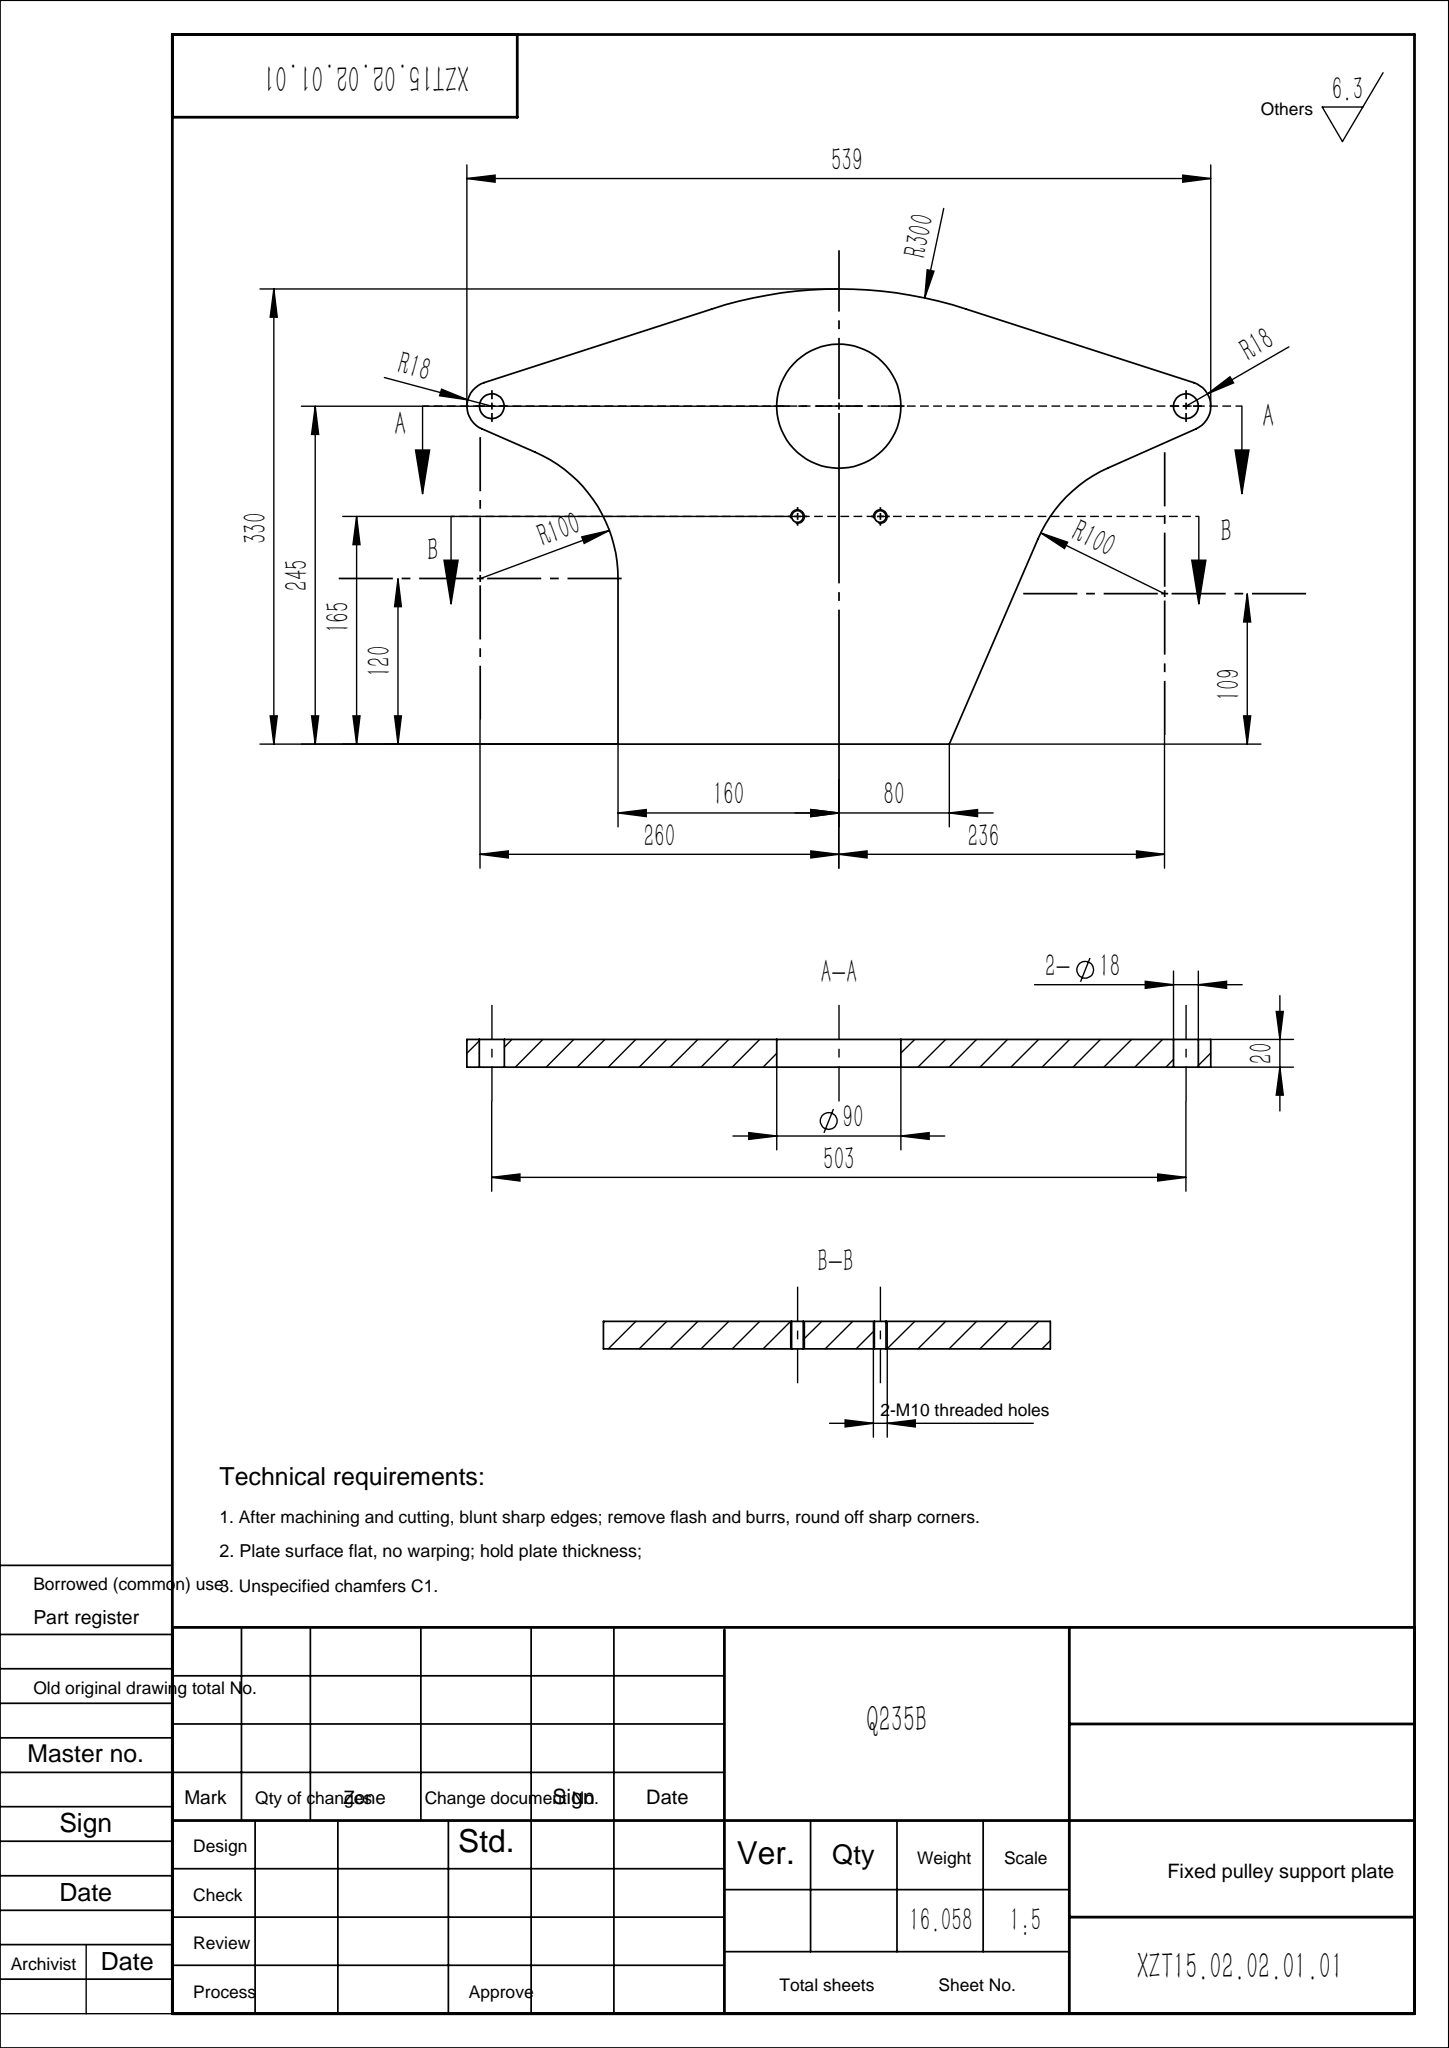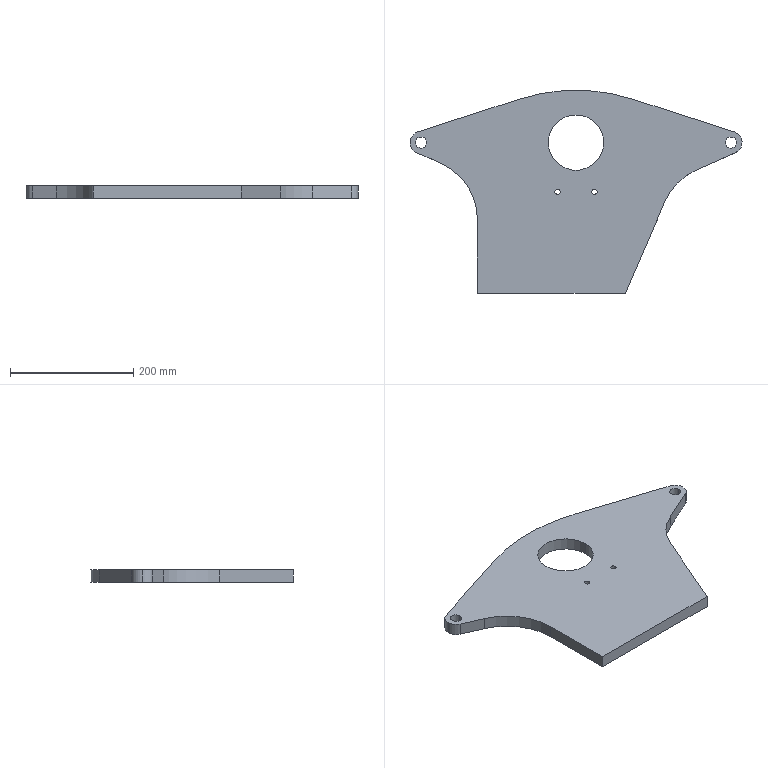Part | SolidWorks | features Extrusion 1, HoleWzd 1 | 1 solid | 25 faces | box 539 x 330 x 20 mm | volume 2045652 mm3 | cylinder 16 | plane 9 | commonest cylinder face diameters 8.5 x4 18 x4 36 x3 90 x2 200 x2 600 x1
STEP:
#1=CARTESIAN_POINT('',(-25.75,165.,-10.));
#2=VERTEX_POINT('',#1);
#3=CARTESIAN_POINT('',(-34.25,165.,-10.));
#4=VERTEX_POINT('',#3);
#5=CARTESIAN_POINT('',(-30.,165.,-10.));
#6=DIRECTION('',(0.,0.,-1.));
#7=DIRECTION('',(-1.,0.,0.));
#8=AXIS2_PLACEMENT_3D('',#5,#6,#7);
#9=CIRCLE('',#8,4.25);
#10=EDGE_CURVE('',#2,#4,#9,.T.);
#11=ORIENTED_EDGE('',*,*,#10,.T.);
#12=CARTESIAN_POINT('',(-34.25,165.,10.));
#13=VERTEX_POINT('',#12);
#14=CARTESIAN_POINT('',(-34.25,165.,10.));
#15=DIRECTION('',(0.,0.,1.));
#16=VECTOR('',#15,1000.);
#17=LINE('',#14,#16);
#18=EDGE_CURVE('',#4,#13,#17,.T.);
#19=ORIENTED_EDGE('',*,*,#18,.T.);
#20=CARTESIAN_POINT('',(-25.75,165.,10.));
#21=VERTEX_POINT('',#20);
#22=CARTESIAN_POINT('',(-30.,165.,10.));
#23=DIRECTION('',(0.,0.,1.));
#24=DIRECTION('',(1.,0.,0.));
#25=AXIS2_PLACEMENT_3D('',#22,#23,#24);
#26=CIRCLE('',#25,4.25);
#27=EDGE_CURVE('',#13,#21,#26,.T.);
#28=ORIENTED_EDGE('',*,*,#27,.T.);
#29=CARTESIAN_POINT('',(-25.75,165.,10.));
#30=DIRECTION('',(0.,0.,1.));
#31=VECTOR('',#30,1000.);
#32=LINE('',#29,#31);
#33=EDGE_CURVE('',#2,#21,#32,.T.);
#34=ORIENTED_EDGE('',*,*,#33,.F.);
#35=EDGE_LOOP('',(#11,#19,#28,#34));
#36=FACE_OUTER_BOUND('',#35,.T.);
#37=CARTESIAN_POINT('',(-30.,165.,10.));
#38=DIRECTION('',(0.,0.,1.));
#39=DIRECTION('',(1.,0.,0.));
#40=AXIS2_PLACEMENT_3D('',#37,#38,#39);
#41=CYLINDRICAL_SURFACE('',#40,4.25);
#42=ADVANCED_FACE('',(#36),#41,.F.);
#43=CARTESIAN_POINT('',(34.25,165.,-10.));
#44=VERTEX_POINT('',#43);
#45=CARTESIAN_POINT('',(25.75,165.,-10.));
#46=VERTEX_POINT('',#45);
#47=CARTESIAN_POINT('',(30.,165.,-10.));
#48=DIRECTION('',(0.,0.,-1.));
#49=DIRECTION('',(-1.,0.,0.));
#50=AXIS2_PLACEMENT_3D('',#47,#48,#49);
#51=CIRCLE('',#50,4.25);
#52=EDGE_CURVE('',#44,#46,#51,.T.);
#53=ORIENTED_EDGE('',*,*,#52,.T.);
#54=CARTESIAN_POINT('',(25.75,165.,10.));
#55=VERTEX_POINT('',#54);
#56=CARTESIAN_POINT('',(25.75,165.,10.));
#57=DIRECTION('',(0.,0.,1.));
#58=VECTOR('',#57,1000.);
#59=LINE('',#56,#58);
#60=EDGE_CURVE('',#46,#55,#59,.T.);
#61=ORIENTED_EDGE('',*,*,#60,.T.);
#62=CARTESIAN_POINT('',(34.25,165.,10.));
#63=VERTEX_POINT('',#62);
#64=CARTESIAN_POINT('',(30.,165.,10.));
#65=DIRECTION('',(0.,0.,1.));
#66=DIRECTION('',(1.,0.,0.));
#67=AXIS2_PLACEMENT_3D('',#64,#65,#66);
#68=CIRCLE('',#67,4.25);
#69=EDGE_CURVE('',#55,#63,#68,.T.);
#70=ORIENTED_EDGE('',*,*,#69,.T.);
#71=CARTESIAN_POINT('',(34.25,165.,10.));
#72=DIRECTION('',(0.,0.,1.));
#73=VECTOR('',#72,1000.);
#74=LINE('',#71,#73);
#75=EDGE_CURVE('',#44,#63,#74,.T.);
#76=ORIENTED_EDGE('',*,*,#75,.F.);
#77=EDGE_LOOP('',(#53,#61,#70,#76));
#78=FACE_OUTER_BOUND('',#77,.T.);
#79=CARTESIAN_POINT('',(30.,165.,10.));
#80=DIRECTION('',(0.,0.,1.));
#81=DIRECTION('',(1.,0.,0.));
#82=AXIS2_PLACEMENT_3D('',#79,#80,#81);
#83=CYLINDRICAL_SURFACE('',#82,4.25);
#84=ADVANCED_FACE('',(#78),#83,.F.);
#85=CARTESIAN_POINT('',(-260.5,245.,10.));
#86=VERTEX_POINT('',#85);
#87=CARTESIAN_POINT('',(-242.5,245.,10.));
#88=VERTEX_POINT('',#87);
#89=CARTESIAN_POINT('',(-251.5,245.,10.));
#90=DIRECTION('',(0.,0.,1.));
#91=DIRECTION('',(1.,0.,0.));
#92=AXIS2_PLACEMENT_3D('',#89,#90,#91);
#93=CIRCLE('',#92,9.);
#94=EDGE_CURVE('',#86,#88,#93,.T.);
#95=ORIENTED_EDGE('',*,*,#94,.T.);
#96=CARTESIAN_POINT('',(-242.5,245.,-10.));
#97=VERTEX_POINT('',#96);
#98=CARTESIAN_POINT('',(-242.5,245.,10.));
#99=DIRECTION('',(0.,0.,-1.));
#100=VECTOR('',#99,1000.);
#101=LINE('',#98,#100);
#102=EDGE_CURVE('',#88,#97,#101,.T.);
#103=ORIENTED_EDGE('',*,*,#102,.T.);
#104=CARTESIAN_POINT('',(-260.5,245.,-10.));
#105=VERTEX_POINT('',#104);
#106=CARTESIAN_POINT('',(-251.5,245.,-10.));
#107=DIRECTION('',(0.,0.,1.));
#108=DIRECTION('',(1.,0.,0.));
#109=AXIS2_PLACEMENT_3D('',#106,#107,#108);
#110=CIRCLE('',#109,9.);
#111=EDGE_CURVE('',#105,#97,#110,.T.);
#112=ORIENTED_EDGE('',*,*,#111,.F.);
#113=CARTESIAN_POINT('',(-260.5,245.,10.));
#114=DIRECTION('',(0.,0.,-1.));
#115=VECTOR('',#114,1000.);
#116=LINE('',#113,#115);
#117=EDGE_CURVE('',#86,#105,#116,.T.);
#118=ORIENTED_EDGE('',*,*,#117,.F.);
#119=EDGE_LOOP('',(#95,#103,#112,#118));
#120=FACE_OUTER_BOUND('',#119,.T.);
#121=CARTESIAN_POINT('',(-251.5,245.,10.));
#122=DIRECTION('',(0.,0.,-1.));
#123=DIRECTION('',(-1.,0.,0.));
#124=AXIS2_PLACEMENT_3D('',#121,#122,#123);
#125=CYLINDRICAL_SURFACE('',#124,9.);
#126=ADVANCED_FACE('',(#120),#125,.F.);
#127=CARTESIAN_POINT('',(242.5,245.,10.));
#128=VERTEX_POINT('',#127);
#129=CARTESIAN_POINT('',(260.5,245.,10.));
#130=VERTEX_POINT('',#129);
#131=CARTESIAN_POINT('',(251.5,245.,10.));
#132=DIRECTION('',(0.,0.,1.));
#133=DIRECTION('',(1.,0.,0.));
#134=AXIS2_PLACEMENT_3D('',#131,#132,#133);
#135=CIRCLE('',#134,9.);
#136=EDGE_CURVE('',#128,#130,#135,.T.);
#137=ORIENTED_EDGE('',*,*,#136,.T.);
#138=CARTESIAN_POINT('',(260.5,245.,-10.));
#139=VERTEX_POINT('',#138);
#140=CARTESIAN_POINT('',(260.5,245.,10.));
#141=DIRECTION('',(0.,0.,-1.));
#142=VECTOR('',#141,1000.);
#143=LINE('',#140,#142);
#144=EDGE_CURVE('',#130,#139,#143,.T.);
#145=ORIENTED_EDGE('',*,*,#144,.T.);
#146=CARTESIAN_POINT('',(242.5,245.,-10.));
#147=VERTEX_POINT('',#146);
#148=CARTESIAN_POINT('',(251.5,245.,-10.));
#149=DIRECTION('',(0.,0.,1.));
#150=DIRECTION('',(1.,0.,0.));
#151=AXIS2_PLACEMENT_3D('',#148,#149,#150);
#152=CIRCLE('',#151,9.);
#153=EDGE_CURVE('',#147,#139,#152,.T.);
#154=ORIENTED_EDGE('',*,*,#153,.F.);
#155=CARTESIAN_POINT('',(242.5,245.,10.));
#156=DIRECTION('',(0.,0.,-1.));
#157=VECTOR('',#156,1000.);
#158=LINE('',#155,#157);
#159=EDGE_CURVE('',#128,#147,#158,.T.);
#160=ORIENTED_EDGE('',*,*,#159,.F.);
#161=EDGE_LOOP('',(#137,#145,#154,#160));
#162=FACE_OUTER_BOUND('',#161,.T.);
#163=CARTESIAN_POINT('',(251.5,245.,10.));
#164=DIRECTION('',(0.,0.,-1.));
#165=DIRECTION('',(-1.,0.,0.));
#166=AXIS2_PLACEMENT_3D('',#163,#164,#165);
#167=CYLINDRICAL_SURFACE('',#166,9.);
#168=ADVANCED_FACE('',(#162),#167,.F.);
#169=CARTESIAN_POINT('',(-45.,245.,10.));
#170=VERTEX_POINT('',#169);
#171=CARTESIAN_POINT('',(45.,245.,10.));
#172=VERTEX_POINT('',#171);
#173=CARTESIAN_POINT('',(0.,245.,10.));
#174=DIRECTION('',(0.,0.,1.));
#175=DIRECTION('',(1.,0.,0.));
#176=AXIS2_PLACEMENT_3D('',#173,#174,#175);
#177=CIRCLE('',#176,45.);
#178=EDGE_CURVE('',#170,#172,#177,.T.);
#179=ORIENTED_EDGE('',*,*,#178,.T.);
#180=CARTESIAN_POINT('',(45.,245.,-10.));
#181=VERTEX_POINT('',#180);
#182=CARTESIAN_POINT('',(45.,245.,10.));
#183=DIRECTION('',(0.,0.,-1.));
#184=VECTOR('',#183,1000.);
#185=LINE('',#182,#184);
#186=EDGE_CURVE('',#172,#181,#185,.T.);
#187=ORIENTED_EDGE('',*,*,#186,.T.);
#188=CARTESIAN_POINT('',(-45.,245.,-10.));
#189=VERTEX_POINT('',#188);
#190=CARTESIAN_POINT('',(0.,245.,-10.));
#191=DIRECTION('',(0.,0.,1.));
#192=DIRECTION('',(1.,0.,0.));
#193=AXIS2_PLACEMENT_3D('',#190,#191,#192);
#194=CIRCLE('',#193,45.);
#195=EDGE_CURVE('',#189,#181,#194,.T.);
#196=ORIENTED_EDGE('',*,*,#195,.F.);
#197=CARTESIAN_POINT('',(-45.,245.,10.));
#198=DIRECTION('',(0.,0.,-1.));
#199=VECTOR('',#198,1000.);
#200=LINE('',#197,#199);
#201=EDGE_CURVE('',#170,#189,#200,.T.);
#202=ORIENTED_EDGE('',*,*,#201,.F.);
#203=EDGE_LOOP('',(#179,#187,#196,#202));
#204=FACE_OUTER_BOUND('',#203,.T.);
#205=CARTESIAN_POINT('',(0.,245.,10.));
#206=DIRECTION('',(0.,0.,-1.));
#207=DIRECTION('',(-1.,0.,0.));
#208=AXIS2_PLACEMENT_3D('',#205,#206,#207);
#209=CYLINDRICAL_SURFACE('',#208,45.);
#210=ADVANCED_FACE('',(#204),#209,.F.);
#211=CARTESIAN_POINT('',(-269.5,245.,10.));
#212=VERTEX_POINT('',#211);
#213=CARTESIAN_POINT('',(-258.686,228.497,10.));
#214=VERTEX_POINT('',#213);
#215=CARTESIAN_POINT('',(-251.5,245.,10.));
#216=DIRECTION('',(0.,0.,1.));
#217=DIRECTION('',(-1.,0.,0.));
#218=AXIS2_PLACEMENT_3D('',#215,#216,#217);
#219=CIRCLE('',#218,18.);
#220=EDGE_CURVE('',#212,#214,#219,.T.);
#221=ORIENTED_EDGE('',*,*,#220,.F.);
#222=CARTESIAN_POINT('',(-269.5,245.,-10.));
#223=VERTEX_POINT('',#222);
#224=CARTESIAN_POINT('',(-269.5,245.,10.));
#225=DIRECTION('',(0.,0.,-1.));
#226=VECTOR('',#225,1000.);
#227=LINE('',#224,#226);
#228=EDGE_CURVE('',#212,#223,#227,.T.);
#229=ORIENTED_EDGE('',*,*,#228,.T.);
#230=CARTESIAN_POINT('',(-258.686,228.497,-10.));
#231=VERTEX_POINT('',#230);
#232=CARTESIAN_POINT('',(-251.5,245.,-10.));
#233=DIRECTION('',(0.,0.,1.));
#234=DIRECTION('',(-1.,0.,0.));
#235=AXIS2_PLACEMENT_3D('',#232,#233,#234);
#236=CIRCLE('',#235,18.);
#237=EDGE_CURVE('',#223,#231,#236,.T.);
#238=ORIENTED_EDGE('',*,*,#237,.T.);
#239=CARTESIAN_POINT('',(-258.686,228.497,10.));
#240=DIRECTION('',(0.,0.,-1.));
#241=VECTOR('',#240,1000.);
#242=LINE('',#239,#241);
#243=EDGE_CURVE('',#214,#231,#242,.T.);
#244=ORIENTED_EDGE('',*,*,#243,.F.);
#245=EDGE_LOOP('',(#221,#229,#238,#244));
#246=FACE_OUTER_BOUND('',#245,.T.);
#247=CARTESIAN_POINT('',(-251.5,245.,10.));
#248=DIRECTION('',(0.,0.,-1.));
#249=DIRECTION('',(-1.,0.,0.));
#250=AXIS2_PLACEMENT_3D('',#247,#248,#249);
#251=CYLINDRICAL_SURFACE('',#250,18.);
#252=ADVANCED_FACE('',(#246),#251,.T.);
#253=CARTESIAN_POINT('',(-160.,0.,10.));
#254=VERTEX_POINT('',#253);
#255=CARTESIAN_POINT('',(80.,0.,10.));
#256=VERTEX_POINT('',#255);
#257=CARTESIAN_POINT('',(0.,0.,10.));
#258=DIRECTION('',(1.,0.,0.));
#259=VECTOR('',#258,1000.);
#260=LINE('',#257,#259);
#261=EDGE_CURVE('',#254,#256,#260,.T.);
#262=ORIENTED_EDGE('',*,*,#261,.T.);
#263=CARTESIAN_POINT('',(144.195,148.647,10.));
#264=VERTEX_POINT('',#263);
#265=CARTESIAN_POINT('',(80.,0.,10.));
#266=DIRECTION('',(0.3965,0.918,0.));
#267=VECTOR('',#266,1000.);
#268=LINE('',#265,#267);
#269=EDGE_CURVE('',#256,#264,#268,.T.);
#270=ORIENTED_EDGE('',*,*,#269,.T.);
#271=CARTESIAN_POINT('',(195.408,200.391,10.));
#272=VERTEX_POINT('',#271);
#273=CARTESIAN_POINT('',(236.,109.,10.));
#274=DIRECTION('',(0.,0.,-1.));
#275=DIRECTION('',(-1.,0.,0.));
#276=AXIS2_PLACEMENT_3D('',#273,#274,#275);
#277=CIRCLE('',#276,100.);
#278=EDGE_CURVE('',#264,#272,#277,.T.);
#279=ORIENTED_EDGE('',*,*,#278,.T.);
#280=CARTESIAN_POINT('',(258.807,228.55,10.));
#281=VERTEX_POINT('',#280);
#282=CARTESIAN_POINT('',(195.408,200.391,10.));
#283=DIRECTION('',(0.9139,0.4059,0.));
#284=VECTOR('',#283,1000.);
#285=LINE('',#282,#284);
#286=EDGE_CURVE('',#272,#281,#285,.T.);
#287=ORIENTED_EDGE('',*,*,#286,.T.);
#288=CARTESIAN_POINT('',(257.043,262.125,10.));
#289=VERTEX_POINT('',#288);
#290=CARTESIAN_POINT('',(251.5,245.,10.));
#291=DIRECTION('',(0.,0.,1.));
#292=DIRECTION('',(1.,0.,0.));
#293=AXIS2_PLACEMENT_3D('',#290,#291,#292);
#294=CIRCLE('',#293,18.);
#295=EDGE_CURVE('',#281,#289,#294,.T.);
#296=ORIENTED_EDGE('',*,*,#295,.T.);
#297=CARTESIAN_POINT('',(92.383,315.421,10.));
#298=VERTEX_POINT('',#297);
#299=CARTESIAN_POINT('',(257.043,262.125,10.));
#300=DIRECTION('',(-0.9514,0.3079,0.));
#301=VECTOR('',#300,1000.);
#302=LINE('',#299,#301);
#303=EDGE_CURVE('',#289,#298,#302,.T.);
#304=ORIENTED_EDGE('',*,*,#303,.T.);
#305=CARTESIAN_POINT('',(-92.383,315.421,10.));
#306=VERTEX_POINT('',#305);
#307=CARTESIAN_POINT('',(0.,30.,10.));
#308=DIRECTION('',(0.,0.,1.));
#309=DIRECTION('',(-1.,0.,0.));
#310=AXIS2_PLACEMENT_3D('',#307,#308,#309);
#311=CIRCLE('',#310,300.);
#312=EDGE_CURVE('',#298,#306,#311,.T.);
#313=ORIENTED_EDGE('',*,*,#312,.T.);
#314=CARTESIAN_POINT('',(-257.043,262.125,10.));
#315=VERTEX_POINT('',#314);
#316=CARTESIAN_POINT('',(-257.043,262.125,10.));
#317=DIRECTION('',(-0.9514,-0.3079,0.));
#318=VECTOR('',#317,1000.);
#319=LINE('',#316,#318);
#320=EDGE_CURVE('',#306,#315,#319,.T.);
#321=ORIENTED_EDGE('',*,*,#320,.T.);
#322=CARTESIAN_POINT('',(-251.5,245.,10.));
#323=DIRECTION('',(0.,0.,1.));
#324=DIRECTION('',(-1.,0.,0.));
#325=AXIS2_PLACEMENT_3D('',#322,#323,#324);
#326=CIRCLE('',#325,18.);
#327=EDGE_CURVE('',#315,#212,#326,.T.);
#328=ORIENTED_EDGE('',*,*,#327,.T.);
#329=ORIENTED_EDGE('',*,*,#220,.T.);
#330=CARTESIAN_POINT('',(-220.077,211.685,10.));
#331=VERTEX_POINT('',#330);
#332=CARTESIAN_POINT('',(-220.077,211.685,10.));
#333=DIRECTION('',(0.9169,-0.3992,0.));
#334=VECTOR('',#333,1000.);
#335=LINE('',#332,#334);
#336=EDGE_CURVE('',#214,#331,#335,.T.);
#337=ORIENTED_EDGE('',*,*,#336,.T.);
#338=CARTESIAN_POINT('',(-160.,120.,10.));
#339=VERTEX_POINT('',#338);
#340=CARTESIAN_POINT('',(-260.,120.,10.));
#341=DIRECTION('',(0.,0.,-1.));
#342=DIRECTION('',(1.,0.,0.));
#343=AXIS2_PLACEMENT_3D('',#340,#341,#342);
#344=CIRCLE('',#343,100.);
#345=EDGE_CURVE('',#331,#339,#344,.T.);
#346=ORIENTED_EDGE('',*,*,#345,.T.);
#347=CARTESIAN_POINT('',(-160.,0.,10.));
#348=DIRECTION('',(0.,-1.,0.));
#349=VECTOR('',#348,1000.);
#350=LINE('',#347,#349);
#351=EDGE_CURVE('',#339,#254,#350,.T.);
#352=ORIENTED_EDGE('',*,*,#351,.T.);
#353=EDGE_LOOP('',(#262,#270,#279,#287,#296,#304,#313,#321,#328,#329,#337,#346,#352));
#354=FACE_OUTER_BOUND('',#353,.T.);
#355=ORIENTED_EDGE('',*,*,#178,.F.);
#356=CARTESIAN_POINT('',(0.,245.,10.));
#357=DIRECTION('',(0.,0.,1.));
#358=DIRECTION('',(1.,0.,0.));
#359=AXIS2_PLACEMENT_3D('',#356,#357,#358);
#360=CIRCLE('',#359,45.);
#361=EDGE_CURVE('',#172,#170,#360,.T.);
#362=ORIENTED_EDGE('',*,*,#361,.F.);
#363=EDGE_LOOP('',(#355,#362));
#364=FACE_BOUND('',#363,.T.);
#365=ORIENTED_EDGE('',*,*,#136,.F.);
#366=CARTESIAN_POINT('',(251.5,245.,10.));
#367=DIRECTION('',(0.,0.,1.));
#368=DIRECTION('',(1.,0.,0.));
#369=AXIS2_PLACEMENT_3D('',#366,#367,#368);
#370=CIRCLE('',#369,9.);
#371=EDGE_CURVE('',#130,#128,#370,.T.);
#372=ORIENTED_EDGE('',*,*,#371,.F.);
#373=EDGE_LOOP('',(#365,#372));
#374=FACE_BOUND('',#373,.T.);
#375=ORIENTED_EDGE('',*,*,#94,.F.);
#376=CARTESIAN_POINT('',(-251.5,245.,10.));
#377=DIRECTION('',(0.,0.,1.));
#378=DIRECTION('',(1.,0.,0.));
#379=AXIS2_PLACEMENT_3D('',#376,#377,#378);
#380=CIRCLE('',#379,9.);
#381=EDGE_CURVE('',#88,#86,#380,.T.);
#382=ORIENTED_EDGE('',*,*,#381,.F.);
#383=EDGE_LOOP('',(#375,#382));
#384=FACE_BOUND('',#383,.T.);
#385=CARTESIAN_POINT('',(30.,165.,10.));
#386=DIRECTION('',(0.,0.,1.));
#387=DIRECTION('',(1.,0.,0.));
#388=AXIS2_PLACEMENT_3D('',#385,#386,#387);
#389=CIRCLE('',#388,4.25);
#390=EDGE_CURVE('',#63,#55,#389,.T.);
#391=ORIENTED_EDGE('',*,*,#390,.F.);
#392=ORIENTED_EDGE('',*,*,#69,.F.);
#393=EDGE_LOOP('',(#391,#392));
#394=FACE_BOUND('',#393,.T.);
#395=CARTESIAN_POINT('',(-30.,165.,10.));
#396=DIRECTION('',(0.,0.,1.));
#397=DIRECTION('',(1.,0.,0.));
#398=AXIS2_PLACEMENT_3D('',#395,#396,#397);
#399=CIRCLE('',#398,4.25);
#400=EDGE_CURVE('',#21,#13,#399,.T.);
#401=ORIENTED_EDGE('',*,*,#400,.F.);
#402=ORIENTED_EDGE('',*,*,#27,.F.);
#403=EDGE_LOOP('',(#401,#402));
#404=FACE_BOUND('',#403,.T.);
#405=CARTESIAN_POINT('',(236.,109.,10.));
#406=DIRECTION('',(0.,0.,-1.));
#407=DIRECTION('',(-1.,0.,0.));
#408=AXIS2_PLACEMENT_3D('',#405,#406,#407);
#409=PLANE('',#408);
#410=ADVANCED_FACE('',(#354,#364,#374,#384,#394,#404),#409,.F.);
#411=ORIENTED_EDGE('',*,*,#10,.F.);
#412=CARTESIAN_POINT('',(-30.,165.,-10.));
#413=DIRECTION('',(0.,0.,-1.));
#414=DIRECTION('',(-1.,0.,0.));
#415=AXIS2_PLACEMENT_3D('',#412,#413,#414);
#416=CIRCLE('',#415,4.25);
#417=EDGE_CURVE('',#4,#2,#416,.T.);
#418=ORIENTED_EDGE('',*,*,#417,.F.);
#419=EDGE_LOOP('',(#411,#418));
#420=FACE_BOUND('',#419,.T.);
#421=ORIENTED_EDGE('',*,*,#52,.F.);
#422=CARTESIAN_POINT('',(30.,165.,-10.));
#423=DIRECTION('',(0.,0.,-1.));
#424=DIRECTION('',(-1.,0.,0.));
#425=AXIS2_PLACEMENT_3D('',#422,#423,#424);
#426=CIRCLE('',#425,4.25);
#427=EDGE_CURVE('',#46,#44,#426,.T.);
#428=ORIENTED_EDGE('',*,*,#427,.F.);
#429=EDGE_LOOP('',(#421,#428));
#430=FACE_BOUND('',#429,.T.);
#431=ORIENTED_EDGE('',*,*,#153,.T.);
#432=CARTESIAN_POINT('',(251.5,245.,-10.));
#433=DIRECTION('',(0.,0.,1.));
#434=DIRECTION('',(1.,0.,0.));
#435=AXIS2_PLACEMENT_3D('',#432,#433,#434);
#436=CIRCLE('',#435,9.);
#437=EDGE_CURVE('',#139,#147,#436,.T.);
#438=ORIENTED_EDGE('',*,*,#437,.T.);
#439=EDGE_LOOP('',(#431,#438));
#440=FACE_BOUND('',#439,.T.);
#441=CARTESIAN_POINT('',(80.,0.,-10.));
#442=VERTEX_POINT('',#441);
#443=CARTESIAN_POINT('',(144.195,148.647,-10.));
#444=VERTEX_POINT('',#443);
#445=CARTESIAN_POINT('',(80.,0.,-10.));
#446=DIRECTION('',(0.3965,0.918,0.));
#447=VECTOR('',#446,1000.);
#448=LINE('',#445,#447);
#449=EDGE_CURVE('',#442,#444,#448,.T.);
#450=ORIENTED_EDGE('',*,*,#449,.F.);
#451=CARTESIAN_POINT('',(-160.,0.,-10.));
#452=VERTEX_POINT('',#451);
#453=CARTESIAN_POINT('',(0.,0.,-10.));
#454=DIRECTION('',(1.,0.,0.));
#455=VECTOR('',#454,1000.);
#456=LINE('',#453,#455);
#457=EDGE_CURVE('',#452,#442,#456,.T.);
#458=ORIENTED_EDGE('',*,*,#457,.F.);
#459=CARTESIAN_POINT('',(-160.,120.,-10.));
#460=VERTEX_POINT('',#459);
#461=CARTESIAN_POINT('',(-160.,0.,-10.));
#462=DIRECTION('',(0.,-1.,0.));
#463=VECTOR('',#462,1000.);
#464=LINE('',#461,#463);
#465=EDGE_CURVE('',#460,#452,#464,.T.);
#466=ORIENTED_EDGE('',*,*,#465,.F.);
#467=CARTESIAN_POINT('',(-220.077,211.685,-10.));
#468=VERTEX_POINT('',#467);
#469=CARTESIAN_POINT('',(-260.,120.,-10.));
#470=DIRECTION('',(0.,0.,-1.));
#471=DIRECTION('',(1.,0.,0.));
#472=AXIS2_PLACEMENT_3D('',#469,#470,#471);
#473=CIRCLE('',#472,100.);
#474=EDGE_CURVE('',#468,#460,#473,.T.);
#475=ORIENTED_EDGE('',*,*,#474,.F.);
#476=CARTESIAN_POINT('',(-220.077,211.685,-10.));
#477=DIRECTION('',(0.9169,-0.3992,0.));
#478=VECTOR('',#477,1000.);
#479=LINE('',#476,#478);
#480=EDGE_CURVE('',#231,#468,#479,.T.);
#481=ORIENTED_EDGE('',*,*,#480,.F.);
#482=ORIENTED_EDGE('',*,*,#237,.F.);
#483=CARTESIAN_POINT('',(-257.043,262.125,-10.));
#484=VERTEX_POINT('',#483);
#485=CARTESIAN_POINT('',(-251.5,245.,-10.));
#486=DIRECTION('',(0.,0.,1.));
#487=DIRECTION('',(-1.,0.,0.));
#488=AXIS2_PLACEMENT_3D('',#485,#486,#487);
#489=CIRCLE('',#488,18.);
#490=EDGE_CURVE('',#484,#223,#489,.T.);
#491=ORIENTED_EDGE('',*,*,#490,.F.);
#492=CARTESIAN_POINT('',(-92.383,315.421,-10.));
#493=VERTEX_POINT('',#492);
#494=CARTESIAN_POINT('',(-257.043,262.125,-10.));
#495=DIRECTION('',(-0.9514,-0.3079,0.));
#496=VECTOR('',#495,1000.);
#497=LINE('',#494,#496);
#498=EDGE_CURVE('',#493,#484,#497,.T.);
#499=ORIENTED_EDGE('',*,*,#498,.F.);
#500=CARTESIAN_POINT('',(92.383,315.421,-10.));
#501=VERTEX_POINT('',#500);
#502=CARTESIAN_POINT('',(0.,30.,-10.));
#503=DIRECTION('',(0.,0.,1.));
#504=DIRECTION('',(-1.,0.,0.));
#505=AXIS2_PLACEMENT_3D('',#502,#503,#504);
#506=CIRCLE('',#505,300.);
#507=EDGE_CURVE('',#501,#493,#506,.T.);
#508=ORIENTED_EDGE('',*,*,#507,.F.);
#509=CARTESIAN_POINT('',(257.043,262.125,-10.));
#510=VERTEX_POINT('',#509);
#511=CARTESIAN_POINT('',(257.043,262.125,-10.));
#512=DIRECTION('',(-0.9514,0.3079,0.));
#513=VECTOR('',#512,1000.);
#514=LINE('',#511,#513);
#515=EDGE_CURVE('',#510,#501,#514,.T.);
#516=ORIENTED_EDGE('',*,*,#515,.F.);
#517=CARTESIAN_POINT('',(258.807,228.55,-10.));
#518=VERTEX_POINT('',#517);
#519=CARTESIAN_POINT('',(251.5,245.,-10.));
#520=DIRECTION('',(0.,0.,1.));
#521=DIRECTION('',(1.,0.,0.));
#522=AXIS2_PLACEMENT_3D('',#519,#520,#521);
#523=CIRCLE('',#522,18.);
#524=EDGE_CURVE('',#518,#510,#523,.T.);
#525=ORIENTED_EDGE('',*,*,#524,.F.);
#526=CARTESIAN_POINT('',(195.408,200.391,-10.));
#527=VERTEX_POINT('',#526);
#528=CARTESIAN_POINT('',(195.408,200.391,-10.));
#529=DIRECTION('',(0.9139,0.4059,0.));
#530=VECTOR('',#529,1000.);
#531=LINE('',#528,#530);
#532=EDGE_CURVE('',#527,#518,#531,.T.);
#533=ORIENTED_EDGE('',*,*,#532,.F.);
#534=CARTESIAN_POINT('',(236.,109.,-10.));
#535=DIRECTION('',(0.,0.,-1.));
#536=DIRECTION('',(-1.,0.,0.));
#537=AXIS2_PLACEMENT_3D('',#534,#535,#536);
#538=CIRCLE('',#537,100.);
#539=EDGE_CURVE('',#444,#527,#538,.T.);
#540=ORIENTED_EDGE('',*,*,#539,.F.);
#541=EDGE_LOOP('',(#450,#458,#466,#475,#481,#482,#491,#499,#508,#516,#525,#533,#540));
#542=FACE_OUTER_BOUND('',#541,.T.);
#543=ORIENTED_EDGE('',*,*,#195,.T.);
#544=CARTESIAN_POINT('',(0.,245.,-10.));
#545=DIRECTION('',(0.,0.,1.));
#546=DIRECTION('',(1.,0.,0.));
#547=AXIS2_PLACEMENT_3D('',#544,#545,#546);
#548=CIRCLE('',#547,45.);
#549=EDGE_CURVE('',#181,#189,#548,.T.);
#550=ORIENTED_EDGE('',*,*,#549,.T.);
#551=EDGE_LOOP('',(#543,#550));
#552=FACE_BOUND('',#551,.T.);
#553=ORIENTED_EDGE('',*,*,#111,.T.);
#554=CARTESIAN_POINT('',(-251.5,245.,-10.));
#555=DIRECTION('',(0.,0.,1.));
#556=DIRECTION('',(1.,0.,0.));
#557=AXIS2_PLACEMENT_3D('',#554,#555,#556);
#558=CIRCLE('',#557,9.);
#559=EDGE_CURVE('',#97,#105,#558,.T.);
#560=ORIENTED_EDGE('',*,*,#559,.T.);
#561=EDGE_LOOP('',(#553,#560));
#562=FACE_BOUND('',#561,.T.);
#563=CARTESIAN_POINT('',(236.,109.,-10.));
#564=DIRECTION('',(0.,0.,-1.));
#565=DIRECTION('',(-1.,0.,0.));
#566=AXIS2_PLACEMENT_3D('',#563,#564,#565);
#567=PLANE('',#566);
#568=ADVANCED_FACE('',(#420,#430,#440,#542,#552,#562),#567,.T.);
#569=ORIENTED_EDGE('',*,*,#449,.T.);
#570=CARTESIAN_POINT('',(144.195,148.647,10.));
#571=DIRECTION('',(0.,0.,-1.));
#572=VECTOR('',#571,1000.);
#573=LINE('',#570,#572);
#574=EDGE_CURVE('',#264,#444,#573,.T.);
#575=ORIENTED_EDGE('',*,*,#574,.F.);
#576=ORIENTED_EDGE('',*,*,#269,.F.);
#577=CARTESIAN_POINT('',(80.,0.,10.));
#578=DIRECTION('',(0.,0.,-1.));
#579=VECTOR('',#578,1000.);
#580=LINE('',#577,#579);
#581=EDGE_CURVE('',#256,#442,#580,.T.);
#582=ORIENTED_EDGE('',*,*,#581,.T.);
#583=EDGE_LOOP('',(#569,#575,#576,#582));
#584=FACE_OUTER_BOUND('',#583,.T.);
#585=CARTESIAN_POINT('',(80.,0.,10.));
#586=DIRECTION('',(-0.918,0.3965,0.));
#587=DIRECTION('',(-0.3965,-0.918,0.));
#588=AXIS2_PLACEMENT_3D('',#585,#586,#587);
#589=PLANE('',#588);
#590=ADVANCED_FACE('',(#584),#589,.F.);
#591=ORIENTED_EDGE('',*,*,#539,.T.);
#592=CARTESIAN_POINT('',(195.408,200.391,10.));
#593=DIRECTION('',(0.,0.,-1.));
#594=VECTOR('',#593,1000.);
#595=LINE('',#592,#594);
#596=EDGE_CURVE('',#272,#527,#595,.T.);
#597=ORIENTED_EDGE('',*,*,#596,.F.);
#598=ORIENTED_EDGE('',*,*,#278,.F.);
#599=ORIENTED_EDGE('',*,*,#574,.T.);
#600=EDGE_LOOP('',(#591,#597,#598,#599));
#601=FACE_OUTER_BOUND('',#600,.T.);
#602=CARTESIAN_POINT('',(236.,109.,10.));
#603=DIRECTION('',(0.,0.,-1.));
#604=DIRECTION('',(-1.,0.,0.));
#605=AXIS2_PLACEMENT_3D('',#602,#603,#604);
#606=CYLINDRICAL_SURFACE('',#605,100.);
#607=ADVANCED_FACE('',(#601),#606,.F.);
#608=ORIENTED_EDGE('',*,*,#532,.T.);
#609=CARTESIAN_POINT('',(258.807,228.55,10.));
#610=DIRECTION('',(0.,0.,-1.));
#611=VECTOR('',#610,1000.);
#612=LINE('',#609,#611);
#613=EDGE_CURVE('',#281,#518,#612,.T.);
#614=ORIENTED_EDGE('',*,*,#613,.F.);
#615=ORIENTED_EDGE('',*,*,#286,.F.);
#616=ORIENTED_EDGE('',*,*,#596,.T.);
#617=EDGE_LOOP('',(#608,#614,#615,#616));
#618=FACE_OUTER_BOUND('',#617,.T.);
#619=CARTESIAN_POINT('',(195.408,200.391,10.));
#620=DIRECTION('',(-0.4059,0.9139,0.));
#621=DIRECTION('',(-0.9139,-0.4059,0.));
#622=AXIS2_PLACEMENT_3D('',#619,#620,#621);
#623=PLANE('',#622);
#624=ADVANCED_FACE('',(#618),#623,.F.);
#625=ORIENTED_EDGE('',*,*,#524,.T.);
#626=CARTESIAN_POINT('',(257.043,262.125,10.));
#627=DIRECTION('',(0.,0.,-1.));
#628=VECTOR('',#627,1000.);
#629=LINE('',#626,#628);
#630=EDGE_CURVE('',#289,#510,#629,.T.);
#631=ORIENTED_EDGE('',*,*,#630,.F.);
#632=ORIENTED_EDGE('',*,*,#295,.F.);
#633=ORIENTED_EDGE('',*,*,#613,.T.);
#634=EDGE_LOOP('',(#625,#631,#632,#633));
#635=FACE_OUTER_BOUND('',#634,.T.);
#636=CARTESIAN_POINT('',(251.5,245.,10.));
#637=DIRECTION('',(0.,0.,-1.));
#638=DIRECTION('',(-1.,0.,0.));
#639=AXIS2_PLACEMENT_3D('',#636,#637,#638);
#640=CYLINDRICAL_SURFACE('',#639,18.);
#641=ADVANCED_FACE('',(#635),#640,.T.);
#642=ORIENTED_EDGE('',*,*,#515,.T.);
#643=CARTESIAN_POINT('',(92.383,315.421,10.));
#644=DIRECTION('',(0.,0.,-1.));
#645=VECTOR('',#644,1000.);
#646=LINE('',#643,#645);
#647=EDGE_CURVE('',#298,#501,#646,.T.);
#648=ORIENTED_EDGE('',*,*,#647,.F.);
#649=ORIENTED_EDGE('',*,*,#303,.F.);
#650=ORIENTED_EDGE('',*,*,#630,.T.);
#651=EDGE_LOOP('',(#642,#648,#649,#650));
#652=FACE_OUTER_BOUND('',#651,.T.);
#653=CARTESIAN_POINT('',(257.043,262.125,10.));
#654=DIRECTION('',(-0.3079,-0.9514,0.));
#655=DIRECTION('',(0.9514,-0.3079,0.));
#656=AXIS2_PLACEMENT_3D('',#653,#654,#655);
#657=PLANE('',#656);
#658=ADVANCED_FACE('',(#652),#657,.F.);
#659=ORIENTED_EDGE('',*,*,#507,.T.);
#660=CARTESIAN_POINT('',(-92.383,315.421,10.));
#661=DIRECTION('',(0.,0.,-1.));
#662=VECTOR('',#661,1000.);
#663=LINE('',#660,#662);
#664=EDGE_CURVE('',#306,#493,#663,.T.);
#665=ORIENTED_EDGE('',*,*,#664,.F.);
#666=ORIENTED_EDGE('',*,*,#312,.F.);
#667=ORIENTED_EDGE('',*,*,#647,.T.);
#668=EDGE_LOOP('',(#659,#665,#666,#667));
#669=FACE_OUTER_BOUND('',#668,.T.);
#670=CARTESIAN_POINT('',(0.,30.,10.));
#671=DIRECTION('',(0.,0.,-1.));
#672=DIRECTION('',(-1.,0.,0.));
#673=AXIS2_PLACEMENT_3D('',#670,#671,#672);
#674=CYLINDRICAL_SURFACE('',#673,300.);
#675=ADVANCED_FACE('',(#669),#674,.T.);
#676=ORIENTED_EDGE('',*,*,#498,.T.);
#677=CARTESIAN_POINT('',(-257.043,262.125,10.));
#678=DIRECTION('',(0.,0.,-1.));
#679=VECTOR('',#678,1000.);
#680=LINE('',#677,#679);
#681=EDGE_CURVE('',#315,#484,#680,.T.);
#682=ORIENTED_EDGE('',*,*,#681,.F.);
#683=ORIENTED_EDGE('',*,*,#320,.F.);
#684=ORIENTED_EDGE('',*,*,#664,.T.);
#685=EDGE_LOOP('',(#676,#682,#683,#684));
#686=FACE_OUTER_BOUND('',#685,.T.);
#687=CARTESIAN_POINT('',(-257.043,262.125,10.));
#688=DIRECTION('',(0.3079,-0.9514,0.));
#689=DIRECTION('',(0.9514,0.3079,0.));
#690=AXIS2_PLACEMENT_3D('',#687,#688,#689);
#691=PLANE('',#690);
#692=ADVANCED_FACE('',(#686),#691,.F.);
#693=ORIENTED_EDGE('',*,*,#228,.F.);
#694=ORIENTED_EDGE('',*,*,#327,.F.);
#695=ORIENTED_EDGE('',*,*,#681,.T.);
#696=ORIENTED_EDGE('',*,*,#490,.T.);
#697=EDGE_LOOP('',(#693,#694,#695,#696));
#698=FACE_OUTER_BOUND('',#697,.T.);
#699=CARTESIAN_POINT('',(-251.5,245.,10.));
#700=DIRECTION('',(0.,0.,-1.));
#701=DIRECTION('',(-1.,0.,0.));
#702=AXIS2_PLACEMENT_3D('',#699,#700,#701);
#703=CYLINDRICAL_SURFACE('',#702,18.);
#704=ADVANCED_FACE('',(#698),#703,.T.);
#705=ORIENTED_EDGE('',*,*,#480,.T.);
#706=CARTESIAN_POINT('',(-220.077,211.685,10.));
#707=DIRECTION('',(0.,0.,-1.));
#708=VECTOR('',#707,1000.);
#709=LINE('',#706,#708);
#710=EDGE_CURVE('',#331,#468,#709,.T.);
#711=ORIENTED_EDGE('',*,*,#710,.F.);
#712=ORIENTED_EDGE('',*,*,#336,.F.);
#713=ORIENTED_EDGE('',*,*,#243,.T.);
#714=EDGE_LOOP('',(#705,#711,#712,#713));
#715=FACE_OUTER_BOUND('',#714,.T.);
#716=CARTESIAN_POINT('',(-220.077,211.685,10.));
#717=DIRECTION('',(0.3992,0.9169,0.));
#718=DIRECTION('',(-0.9169,0.3992,0.));
#719=AXIS2_PLACEMENT_3D('',#716,#717,#718);
#720=PLANE('',#719);
#721=ADVANCED_FACE('',(#715),#720,.F.);
#722=ORIENTED_EDGE('',*,*,#474,.T.);
#723=CARTESIAN_POINT('',(-160.,120.,10.));
#724=DIRECTION('',(0.,0.,-1.));
#725=VECTOR('',#724,1000.);
#726=LINE('',#723,#725);
#727=EDGE_CURVE('',#339,#460,#726,.T.);
#728=ORIENTED_EDGE('',*,*,#727,.F.);
#729=ORIENTED_EDGE('',*,*,#345,.F.);
#730=ORIENTED_EDGE('',*,*,#710,.T.);
#731=EDGE_LOOP('',(#722,#728,#729,#730));
#732=FACE_OUTER_BOUND('',#731,.T.);
#733=CARTESIAN_POINT('',(-260.,120.,10.));
#734=DIRECTION('',(0.,0.,-1.));
#735=DIRECTION('',(-1.,0.,0.));
#736=AXIS2_PLACEMENT_3D('',#733,#734,#735);
#737=CYLINDRICAL_SURFACE('',#736,100.);
#738=ADVANCED_FACE('',(#732),#737,.F.);
#739=ORIENTED_EDGE('',*,*,#465,.T.);
#740=CARTESIAN_POINT('',(-160.,0.,10.));
#741=DIRECTION('',(0.,0.,-1.));
#742=VECTOR('',#741,1000.);
#743=LINE('',#740,#742);
#744=EDGE_CURVE('',#254,#452,#743,.T.);
#745=ORIENTED_EDGE('',*,*,#744,.F.);
#746=ORIENTED_EDGE('',*,*,#351,.F.);
#747=ORIENTED_EDGE('',*,*,#727,.T.);
#748=EDGE_LOOP('',(#739,#745,#746,#747));
#749=FACE_OUTER_BOUND('',#748,.T.);
#750=CARTESIAN_POINT('',(-160.,0.,10.));
#751=DIRECTION('',(1.,0.,0.));
#752=DIRECTION('',(0.,1.,0.));
#753=AXIS2_PLACEMENT_3D('',#750,#751,#752);
#754=PLANE('',#753);
#755=ADVANCED_FACE('',(#749),#754,.F.);
#756=ORIENTED_EDGE('',*,*,#457,.T.);
#757=ORIENTED_EDGE('',*,*,#581,.F.);
#758=ORIENTED_EDGE('',*,*,#261,.F.);
#759=ORIENTED_EDGE('',*,*,#744,.T.);
#760=EDGE_LOOP('',(#756,#757,#758,#759));
#761=FACE_OUTER_BOUND('',#760,.T.);
#762=CARTESIAN_POINT('',(0.,0.,10.));
#763=DIRECTION('',(0.,1.,0.));
#764=DIRECTION('',(-1.,0.,0.));
#765=AXIS2_PLACEMENT_3D('',#762,#763,#764);
#766=PLANE('',#765);
#767=ADVANCED_FACE('',(#761),#766,.F.);
#768=ORIENTED_EDGE('',*,*,#186,.F.);
#769=ORIENTED_EDGE('',*,*,#361,.T.);
#770=ORIENTED_EDGE('',*,*,#201,.T.);
#771=ORIENTED_EDGE('',*,*,#549,.F.);
#772=EDGE_LOOP('',(#768,#769,#770,#771));
#773=FACE_OUTER_BOUND('',#772,.T.);
#774=CARTESIAN_POINT('',(0.,245.,10.));
#775=DIRECTION('',(0.,0.,-1.));
#776=DIRECTION('',(-1.,0.,0.));
#777=AXIS2_PLACEMENT_3D('',#774,#775,#776);
#778=CYLINDRICAL_SURFACE('',#777,45.);
#779=ADVANCED_FACE('',(#773),#778,.F.);
#780=ORIENTED_EDGE('',*,*,#144,.F.);
#781=ORIENTED_EDGE('',*,*,#371,.T.);
#782=ORIENTED_EDGE('',*,*,#159,.T.);
#783=ORIENTED_EDGE('',*,*,#437,.F.);
#784=EDGE_LOOP('',(#780,#781,#782,#783));
#785=FACE_OUTER_BOUND('',#784,.T.);
#786=CARTESIAN_POINT('',(251.5,245.,10.));
#787=DIRECTION('',(0.,0.,-1.));
#788=DIRECTION('',(-1.,0.,0.));
#789=AXIS2_PLACEMENT_3D('',#786,#787,#788);
#790=CYLINDRICAL_SURFACE('',#789,9.);
#791=ADVANCED_FACE('',(#785),#790,.F.);
#792=ORIENTED_EDGE('',*,*,#102,.F.);
#793=ORIENTED_EDGE('',*,*,#381,.T.);
#794=ORIENTED_EDGE('',*,*,#117,.T.);
#795=ORIENTED_EDGE('',*,*,#559,.F.);
#796=EDGE_LOOP('',(#792,#793,#794,#795));
#797=FACE_OUTER_BOUND('',#796,.T.);
#798=CARTESIAN_POINT('',(-251.5,245.,10.));
#799=DIRECTION('',(0.,0.,-1.));
#800=DIRECTION('',(-1.,0.,0.));
#801=AXIS2_PLACEMENT_3D('',#798,#799,#800);
#802=CYLINDRICAL_SURFACE('',#801,9.);
#803=ADVANCED_FACE('',(#797),#802,.F.);
#804=ORIENTED_EDGE('',*,*,#60,.F.);
#805=ORIENTED_EDGE('',*,*,#427,.T.);
#806=ORIENTED_EDGE('',*,*,#75,.T.);
#807=ORIENTED_EDGE('',*,*,#390,.T.);
#808=EDGE_LOOP('',(#804,#805,#806,#807));
#809=FACE_OUTER_BOUND('',#808,.T.);
#810=CARTESIAN_POINT('',(30.,165.,10.));
#811=DIRECTION('',(0.,0.,1.));
#812=DIRECTION('',(1.,0.,0.));
#813=AXIS2_PLACEMENT_3D('',#810,#811,#812);
#814=CYLINDRICAL_SURFACE('',#813,4.25);
#815=ADVANCED_FACE('',(#809),#814,.F.);
#816=ORIENTED_EDGE('',*,*,#18,.F.);
#817=ORIENTED_EDGE('',*,*,#417,.T.);
#818=ORIENTED_EDGE('',*,*,#33,.T.);
#819=ORIENTED_EDGE('',*,*,#400,.T.);
#820=EDGE_LOOP('',(#816,#817,#818,#819));
#821=FACE_OUTER_BOUND('',#820,.T.);
#822=CARTESIAN_POINT('',(-30.,165.,10.));
#823=DIRECTION('',(0.,0.,1.));
#824=DIRECTION('',(1.,0.,0.));
#825=AXIS2_PLACEMENT_3D('',#822,#823,#824);
#826=CYLINDRICAL_SURFACE('',#825,4.25);
#827=ADVANCED_FACE('',(#821),#826,.F.);
#828=CLOSED_SHELL('',(#42,#84,#126,#168,#210,#252,#410,#568,#590,#607,#624,#641,#658,#675,#692,#704,#721,#738,#755,#767,#779,#791,#803,#815,#827));
#829=MANIFOLD_SOLID_BREP('',#828);
#830=CARTESIAN_POINT('',(0.,0.,0.));
#831=DIRECTION('',(0.,0.,1.));
#832=DIRECTION('',(1.,0.,0.));
#833=AXIS2_PLACEMENT_3D('',#830,#831,#832);
#834=(LENGTH_UNIT()NAMED_UNIT(*)SI_UNIT(.MILLI.,.METRE.));
#835=UNCERTAINTY_MEASURE_WITH_UNIT(LENGTH_MEASURE(0.00001),#834,'','');
#836=(NAMED_UNIT(*)PLANE_ANGLE_UNIT()SI_UNIT($,.RADIAN.));
#837=(NAMED_UNIT(*)SI_UNIT($,.STERADIAN.)SOLID_ANGLE_UNIT());
#838=(GEOMETRIC_REPRESENTATION_CONTEXT(3)GLOBAL_UNCERTAINTY_ASSIGNED_CONTEXT((#835))GLOBAL_UNIT_ASSIGNED_CONTEXT((#834,#836,#837))REPRESENTATION_CONTEXT('',''));
#839=ADVANCED_BREP_SHAPE_REPRESENTATION('',(#829,#833),#838);